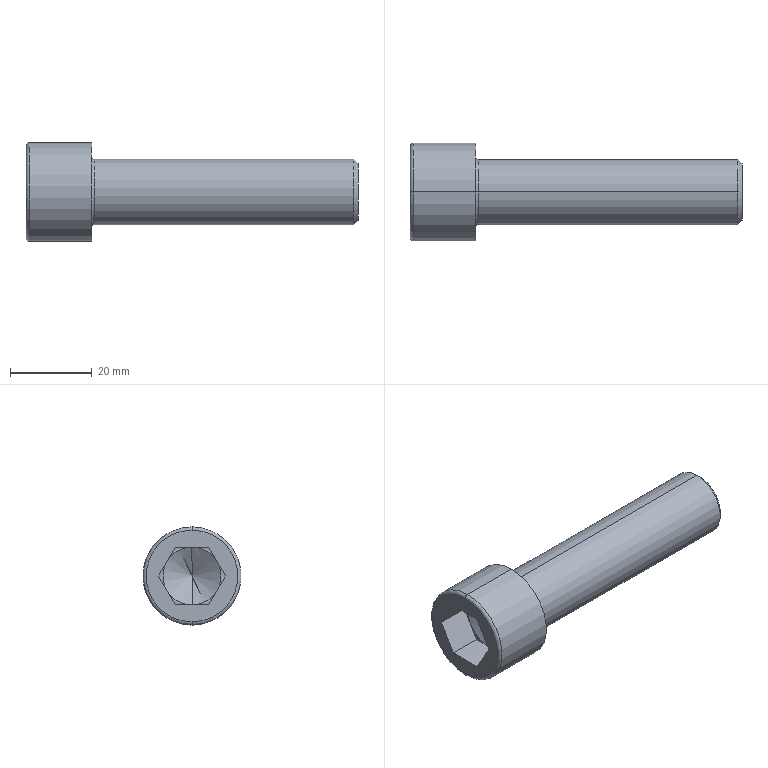Part | STEP file | P-001093_JIS B 1176 M16 x 50 (50) --N | 1 solid | 27 faces | box 81 x 24 x 24 mm | volume 18678 mm3 | plane 15 | cone 4 | torus 4 | cylinder 4 | commonest cylinder face diameters 16 x2 24 x2